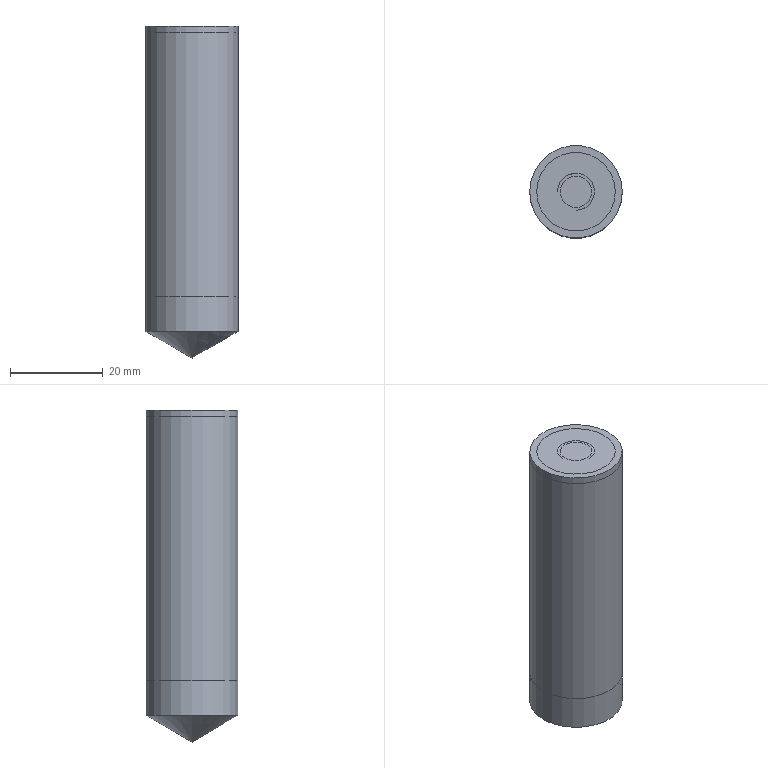Part | STEP file | DP20-1 | 2 solids | 48 faces | box 20 x 20 x 71.774 mm | volume 40454 mm3 | plane 18 | cone 12 | other 12 | cylinder 5 | spline 1 | commonest cylinder face diameters 20 x2 6.8 x1 7.973 x1 8 x1